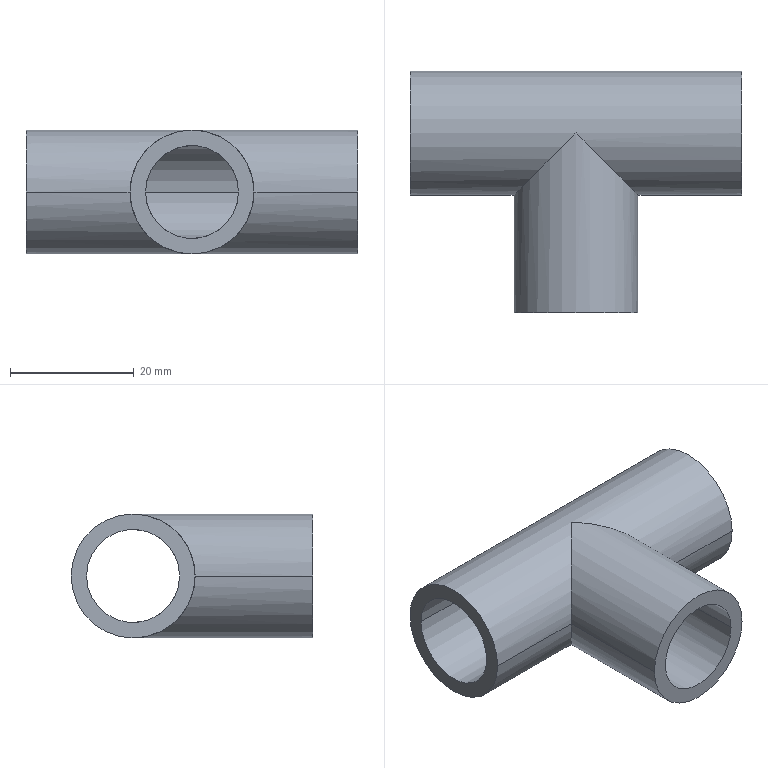Part | SolidWorks | features ICE 2, Sweep 2 | 1 solid | 15 faces | box 53.5 x 39 x 20 mm | volume 9797 mm3 | cylinder 10 | plane 5 | commonest cylinder face diameters 15 x6 20 x4
STEP:
#1=CARTESIAN_POINT('',(-26.75,-7.5,0.));
#2=VERTEX_POINT('',#1);
#3=CARTESIAN_POINT('',(-26.75,7.5,0.));
#4=VERTEX_POINT('',#3);
#5=CARTESIAN_POINT('',(-26.75,0.,0.));
#6=DIRECTION('',(1.,0.,0.));
#7=DIRECTION('',(0.,1.,0.));
#8=AXIS2_PLACEMENT_3D('',#5,#6,#7);
#9=CIRCLE('',#8,7.5);
#10=EDGE_CURVE('',#2,#4,#9,.T.);
#11=ORIENTED_EDGE('',*,*,#10,.F.);
#12=CARTESIAN_POINT('',(-7.5,-7.5,0.));
#13=VERTEX_POINT('',#12);
#14=CARTESIAN_POINT('',(-26.75,-7.5,0.));
#15=DIRECTION('',(1.,0.,0.));
#16=VECTOR('',#15,1000.);
#17=LINE('',#14,#16);
#18=EDGE_CURVE('',#2,#13,#17,.T.);
#19=ORIENTED_EDGE('',*,*,#18,.T.);
#20=CARTESIAN_POINT('',(0.,0.,-7.5));
#21=VERTEX_POINT('',#20);
#22=CARTESIAN_POINT('',(-7.5,-7.5,0.));
#23=CARTESIAN_POINT('',(-7.5,-7.5,-4.393));
#24=CARTESIAN_POINT('',(-4.393,-4.393,-7.5));
#25=CARTESIAN_POINT('',(0.,0.,-7.5));
#26=(BOUNDED_CURVE()B_SPLINE_CURVE(3,(#22,#23,#24,#25),.UNSPECIFIED.,.F.,.F.)B_SPLINE_CURVE_WITH_KNOTS((4,4),(3.142,4.712),.UNSPECIFIED.)CURVE()GEOMETRIC_REPRESENTATION_ITEM()RATIONAL_B_SPLINE_CURVE((1.,0.8047,0.8047,1.))REPRESENTATION_ITEM(''));
#27=EDGE_CURVE('',#13,#21,#26,.T.);
#28=ORIENTED_EDGE('',*,*,#27,.T.);
#29=CARTESIAN_POINT('',(-1.,1.,-7.433));
#30=VERTEX_POINT('',#29);
#31=CARTESIAN_POINT('',(0.,0.,-7.5));
#32=CARTESIAN_POINT('',(-0.3346,0.3346,-7.5));
#33=CARTESIAN_POINT('',(-0.6684,0.6684,-7.478));
#34=CARTESIAN_POINT('',(-1.,1.,-7.433));
#35=(BOUNDED_CURVE()B_SPLINE_CURVE(3,(#31,#32,#33,#34),.UNSPECIFIED.,.F.,.F.)B_SPLINE_CURVE_WITH_KNOTS((4,4),(1.571,1.705),.UNSPECIFIED.)CURVE()GEOMETRIC_REPRESENTATION_ITEM()RATIONAL_B_SPLINE_CURVE((1.,0.9985,0.9985,1.))REPRESENTATION_ITEM(''));
#36=EDGE_CURVE('',#21,#30,#35,.T.);
#37=ORIENTED_EDGE('',*,*,#36,.T.);
#38=CARTESIAN_POINT('',(1.,1.,-7.433));
#39=VERTEX_POINT('',#38);
#40=CARTESIAN_POINT('',(-26.75,1.,-7.433));
#41=DIRECTION('',(-1.,0.,0.));
#42=VECTOR('',#41,1000.);
#43=LINE('',#40,#42);
#44=EDGE_CURVE('',#39,#30,#43,.T.);
#45=ORIENTED_EDGE('',*,*,#44,.F.);
#46=CARTESIAN_POINT('',(1.,1.,-7.433));
#47=CARTESIAN_POINT('',(0.6684,0.6684,-7.478));
#48=CARTESIAN_POINT('',(0.3346,0.3346,-7.5));
#49=CARTESIAN_POINT('',(0.,0.,-7.5));
#50=(BOUNDED_CURVE()B_SPLINE_CURVE(3,(#46,#47,#48,#49),.UNSPECIFIED.,.F.,.F.)B_SPLINE_CURVE_WITH_KNOTS((4,4),(1.437,1.571),.UNSPECIFIED.)CURVE()GEOMETRIC_REPRESENTATION_ITEM()RATIONAL_B_SPLINE_CURVE((1.,0.9985,0.9985,1.))REPRESENTATION_ITEM(''));
#51=EDGE_CURVE('',#39,#21,#50,.T.);
#52=ORIENTED_EDGE('',*,*,#51,.T.);
#53=CARTESIAN_POINT('',(7.5,-7.5,0.));
#54=VERTEX_POINT('',#53);
#55=CARTESIAN_POINT('',(0.,0.,-7.5));
#56=CARTESIAN_POINT('',(4.393,-4.393,-7.5));
#57=CARTESIAN_POINT('',(7.5,-7.5,-4.393));
#58=CARTESIAN_POINT('',(7.5,-7.5,0.));
#59=(BOUNDED_CURVE()B_SPLINE_CURVE(3,(#55,#56,#57,#58),.UNSPECIFIED.,.F.,.F.)B_SPLINE_CURVE_WITH_KNOTS((4,4),(4.712,6.283),.UNSPECIFIED.)CURVE()GEOMETRIC_REPRESENTATION_ITEM()RATIONAL_B_SPLINE_CURVE((1.,0.8047,0.8047,1.))REPRESENTATION_ITEM(''));
#60=EDGE_CURVE('',#21,#54,#59,.T.);
#61=ORIENTED_EDGE('',*,*,#60,.T.);
#62=CARTESIAN_POINT('',(26.75,-7.5,0.));
#63=VERTEX_POINT('',#62);
#64=CARTESIAN_POINT('',(-26.75,-7.5,0.));
#65=DIRECTION('',(1.,0.,0.));
#66=VECTOR('',#65,1000.);
#67=LINE('',#64,#66);
#68=EDGE_CURVE('',#54,#63,#67,.T.);
#69=ORIENTED_EDGE('',*,*,#68,.T.);
#70=CARTESIAN_POINT('',(26.75,7.5,0.));
#71=VERTEX_POINT('',#70);
#72=CARTESIAN_POINT('',(26.75,0.,0.));
#73=DIRECTION('',(1.,0.,0.));
#74=DIRECTION('',(0.,1.,0.));
#75=AXIS2_PLACEMENT_3D('',#72,#73,#74);
#76=CIRCLE('',#75,7.5);
#77=EDGE_CURVE('',#63,#71,#76,.T.);
#78=ORIENTED_EDGE('',*,*,#77,.T.);
#79=CARTESIAN_POINT('',(-26.75,7.5,0.));
#80=DIRECTION('',(1.,0.,0.));
#81=VECTOR('',#80,1000.);
#82=LINE('',#79,#81);
#83=EDGE_CURVE('',#4,#71,#82,.T.);
#84=ORIENTED_EDGE('',*,*,#83,.F.);
#85=EDGE_LOOP('',(#11,#19,#28,#37,#45,#52,#61,#69,#78,#84));
#86=FACE_OUTER_BOUND('',#85,.T.);
#87=CARTESIAN_POINT('',(-26.75,0.,0.));
#88=DIRECTION('',(1.,0.,0.));
#89=DIRECTION('',(0.,1.,0.));
#90=AXIS2_PLACEMENT_3D('',#87,#88,#89);
#91=CYLINDRICAL_SURFACE('',#90,7.5);
#92=ADVANCED_FACE('',(#86),#91,.F.);
#93=ORIENTED_EDGE('',*,*,#27,.F.);
#94=CARTESIAN_POINT('',(-7.5,-29.,0.));
#95=VERTEX_POINT('',#94);
#96=CARTESIAN_POINT('',(-7.5,0.,0.));
#97=DIRECTION('',(0.,-1.,0.));
#98=VECTOR('',#97,1000.);
#99=LINE('',#96,#98);
#100=EDGE_CURVE('',#13,#95,#99,.T.);
#101=ORIENTED_EDGE('',*,*,#100,.T.);
#102=CARTESIAN_POINT('',(7.5,-29.,0.));
#103=VERTEX_POINT('',#102);
#104=CARTESIAN_POINT('',(0.,-29.,0.));
#105=DIRECTION('',(0.,-1.,0.));
#106=DIRECTION('',(1.,0.,0.));
#107=AXIS2_PLACEMENT_3D('',#104,#105,#106);
#108=CIRCLE('',#107,7.5);
#109=EDGE_CURVE('',#95,#103,#108,.T.);
#110=ORIENTED_EDGE('',*,*,#109,.T.);
#111=CARTESIAN_POINT('',(7.5,0.,0.));
#112=DIRECTION('',(0.,-1.,0.));
#113=VECTOR('',#112,1000.);
#114=LINE('',#111,#113);
#115=EDGE_CURVE('',#54,#103,#114,.T.);
#116=ORIENTED_EDGE('',*,*,#115,.F.);
#117=ORIENTED_EDGE('',*,*,#60,.F.);
#118=EDGE_LOOP('',(#93,#101,#110,#116,#117));
#119=FACE_OUTER_BOUND('',#118,.T.);
#120=CARTESIAN_POINT('',(0.,0.,0.));
#121=DIRECTION('',(0.,-1.,0.));
#122=DIRECTION('',(1.,0.,0.));
#123=AXIS2_PLACEMENT_3D('',#120,#121,#122);
#124=CYLINDRICAL_SURFACE('',#123,7.5);
#125=ADVANCED_FACE('',(#119),#124,.F.);
#126=CARTESIAN_POINT('',(0.,0.,10.));
#127=VERTEX_POINT('',#126);
#128=CARTESIAN_POINT('',(-10.,-10.,0.));
#129=VERTEX_POINT('',#128);
#130=CARTESIAN_POINT('',(0.,0.,10.));
#131=CARTESIAN_POINT('',(-5.858,-5.858,10.));
#132=CARTESIAN_POINT('',(-10.,-10.,5.858));
#133=CARTESIAN_POINT('',(-10.,-10.,0.));
#134=(BOUNDED_CURVE()B_SPLINE_CURVE(3,(#130,#131,#132,#133),.UNSPECIFIED.,.F.,.F.)B_SPLINE_CURVE_WITH_KNOTS((4,4),(1.571,3.142),.UNSPECIFIED.)CURVE()GEOMETRIC_REPRESENTATION_ITEM()RATIONAL_B_SPLINE_CURVE((1.,0.8047,0.8047,1.))REPRESENTATION_ITEM(''));
#135=EDGE_CURVE('',#127,#129,#134,.T.);
#136=ORIENTED_EDGE('',*,*,#135,.T.);
#137=CARTESIAN_POINT('',(-10.,-29.,0.));
#138=VERTEX_POINT('',#137);
#139=CARTESIAN_POINT('',(-10.,0.,0.));
#140=DIRECTION('',(0.,-1.,0.));
#141=VECTOR('',#140,1000.);
#142=LINE('',#139,#141);
#143=EDGE_CURVE('',#129,#138,#142,.T.);
#144=ORIENTED_EDGE('',*,*,#143,.T.);
#145=CARTESIAN_POINT('',(10.,-29.,0.));
#146=VERTEX_POINT('',#145);
#147=CARTESIAN_POINT('',(0.,-29.,0.));
#148=DIRECTION('',(0.,-1.,0.));
#149=DIRECTION('',(1.,0.,0.));
#150=AXIS2_PLACEMENT_3D('',#147,#148,#149);
#151=CIRCLE('',#150,10.);
#152=EDGE_CURVE('',#146,#138,#151,.T.);
#153=ORIENTED_EDGE('',*,*,#152,.F.);
#154=CARTESIAN_POINT('',(10.,-10.,0.));
#155=VERTEX_POINT('',#154);
#156=CARTESIAN_POINT('',(10.,0.,0.));
#157=DIRECTION('',(0.,-1.,0.));
#158=VECTOR('',#157,1000.);
#159=LINE('',#156,#158);
#160=EDGE_CURVE('',#155,#146,#159,.T.);
#161=ORIENTED_EDGE('',*,*,#160,.F.);
#162=CARTESIAN_POINT('',(10.,-10.,0.));
#163=CARTESIAN_POINT('',(10.,-10.,5.858));
#164=CARTESIAN_POINT('',(5.858,-5.858,10.));
#165=CARTESIAN_POINT('',(0.,0.,10.));
#166=(BOUNDED_CURVE()B_SPLINE_CURVE(3,(#162,#163,#164,#165),.UNSPECIFIED.,.F.,.F.)B_SPLINE_CURVE_WITH_KNOTS((4,4),(0.,1.571),.UNSPECIFIED.)CURVE()GEOMETRIC_REPRESENTATION_ITEM()RATIONAL_B_SPLINE_CURVE((1.,0.8047,0.8047,1.))REPRESENTATION_ITEM(''));
#167=EDGE_CURVE('',#155,#127,#166,.T.);
#168=ORIENTED_EDGE('',*,*,#167,.T.);
#169=EDGE_LOOP('',(#136,#144,#153,#161,#168));
#170=FACE_OUTER_BOUND('',#169,.T.);
#171=CARTESIAN_POINT('',(0.,0.,0.));
#172=DIRECTION('',(0.,-1.,0.));
#173=DIRECTION('',(1.,0.,0.));
#174=AXIS2_PLACEMENT_3D('',#171,#172,#173);
#175=CYLINDRICAL_SURFACE('',#174,10.);
#176=ADVANCED_FACE('',(#170),#175,.T.);
#177=CARTESIAN_POINT('',(-26.75,10.,0.));
#178=VERTEX_POINT('',#177);
#179=CARTESIAN_POINT('',(-26.75,-10.,0.));
#180=VERTEX_POINT('',#179);
#181=CARTESIAN_POINT('',(-26.75,0.,0.));
#182=DIRECTION('',(1.,0.,0.));
#183=DIRECTION('',(0.,1.,0.));
#184=AXIS2_PLACEMENT_3D('',#181,#182,#183);
#185=CIRCLE('',#184,10.);
#186=EDGE_CURVE('',#178,#180,#185,.T.);
#187=ORIENTED_EDGE('',*,*,#186,.T.);
#188=CARTESIAN_POINT('',(-26.75,-10.,0.));
#189=DIRECTION('',(1.,0.,0.));
#190=VECTOR('',#189,1000.);
#191=LINE('',#188,#190);
#192=EDGE_CURVE('',#180,#129,#191,.T.);
#193=ORIENTED_EDGE('',*,*,#192,.T.);
#194=ORIENTED_EDGE('',*,*,#135,.F.);
#195=ORIENTED_EDGE('',*,*,#167,.F.);
#196=CARTESIAN_POINT('',(26.75,-10.,0.));
#197=VERTEX_POINT('',#196);
#198=CARTESIAN_POINT('',(-26.75,-10.,0.));
#199=DIRECTION('',(1.,0.,0.));
#200=VECTOR('',#199,1000.);
#201=LINE('',#198,#200);
#202=EDGE_CURVE('',#155,#197,#201,.T.);
#203=ORIENTED_EDGE('',*,*,#202,.T.);
#204=CARTESIAN_POINT('',(26.75,10.,0.));
#205=VERTEX_POINT('',#204);
#206=CARTESIAN_POINT('',(26.75,0.,0.));
#207=DIRECTION('',(1.,0.,0.));
#208=DIRECTION('',(0.,1.,0.));
#209=AXIS2_PLACEMENT_3D('',#206,#207,#208);
#210=CIRCLE('',#209,10.);
#211=EDGE_CURVE('',#205,#197,#210,.T.);
#212=ORIENTED_EDGE('',*,*,#211,.F.);
#213=CARTESIAN_POINT('',(-26.75,10.,0.));
#214=DIRECTION('',(1.,0.,0.));
#215=VECTOR('',#214,1000.);
#216=LINE('',#213,#215);
#217=EDGE_CURVE('',#178,#205,#216,.T.);
#218=ORIENTED_EDGE('',*,*,#217,.F.);
#219=EDGE_LOOP('',(#187,#193,#194,#195,#203,#212,#218));
#220=FACE_OUTER_BOUND('',#219,.T.);
#221=CARTESIAN_POINT('',(-26.75,0.,0.));
#222=DIRECTION('',(1.,0.,0.));
#223=DIRECTION('',(0.,1.,0.));
#224=AXIS2_PLACEMENT_3D('',#221,#222,#223);
#225=CYLINDRICAL_SURFACE('',#224,10.);
#226=ADVANCED_FACE('',(#220),#225,.T.);
#227=ORIENTED_EDGE('',*,*,#192,.F.);
#228=CARTESIAN_POINT('',(-26.75,0.,0.));
#229=DIRECTION('',(1.,0.,0.));
#230=DIRECTION('',(0.,1.,0.));
#231=AXIS2_PLACEMENT_3D('',#228,#229,#230);
#232=CIRCLE('',#231,10.);
#233=EDGE_CURVE('',#180,#178,#232,.T.);
#234=ORIENTED_EDGE('',*,*,#233,.T.);
#235=ORIENTED_EDGE('',*,*,#217,.T.);
#236=CARTESIAN_POINT('',(26.75,0.,0.));
#237=DIRECTION('',(1.,0.,0.));
#238=DIRECTION('',(0.,1.,0.));
#239=AXIS2_PLACEMENT_3D('',#236,#237,#238);
#240=CIRCLE('',#239,10.);
#241=EDGE_CURVE('',#197,#205,#240,.T.);
#242=ORIENTED_EDGE('',*,*,#241,.F.);
#243=ORIENTED_EDGE('',*,*,#202,.F.);
#244=CARTESIAN_POINT('',(0.,0.,-10.));
#245=VERTEX_POINT('',#244);
#246=CARTESIAN_POINT('',(0.,0.,-10.));
#247=CARTESIAN_POINT('',(5.858,-5.858,-10.));
#248=CARTESIAN_POINT('',(10.,-10.,-5.858));
#249=CARTESIAN_POINT('',(10.,-10.,0.));
#250=(BOUNDED_CURVE()B_SPLINE_CURVE(3,(#246,#247,#248,#249),.UNSPECIFIED.,.F.,.F.)B_SPLINE_CURVE_WITH_KNOTS((4,4),(4.712,6.283),.UNSPECIFIED.)CURVE()GEOMETRIC_REPRESENTATION_ITEM()RATIONAL_B_SPLINE_CURVE((1.,0.8047,0.8047,1.))REPRESENTATION_ITEM(''));
#251=EDGE_CURVE('',#245,#155,#250,.T.);
#252=ORIENTED_EDGE('',*,*,#251,.F.);
#253=CARTESIAN_POINT('',(-10.,-10.,0.));
#254=CARTESIAN_POINT('',(-10.,-10.,-5.858));
#255=CARTESIAN_POINT('',(-5.858,-5.858,-10.));
#256=CARTESIAN_POINT('',(0.,0.,-10.));
#257=(BOUNDED_CURVE()B_SPLINE_CURVE(3,(#253,#254,#255,#256),.UNSPECIFIED.,.F.,.F.)B_SPLINE_CURVE_WITH_KNOTS((4,4),(3.142,4.712),.UNSPECIFIED.)CURVE()GEOMETRIC_REPRESENTATION_ITEM()RATIONAL_B_SPLINE_CURVE((1.,0.8047,0.8047,1.))REPRESENTATION_ITEM(''));
#258=EDGE_CURVE('',#129,#245,#257,.T.);
#259=ORIENTED_EDGE('',*,*,#258,.F.);
#260=EDGE_LOOP('',(#227,#234,#235,#242,#243,#252,#259));
#261=FACE_OUTER_BOUND('',#260,.T.);
#262=CARTESIAN_POINT('',(-26.75,0.,0.));
#263=DIRECTION('',(1.,0.,0.));
#264=DIRECTION('',(0.,1.,0.));
#265=AXIS2_PLACEMENT_3D('',#262,#263,#264);
#266=CYLINDRICAL_SURFACE('',#265,10.);
#267=ADVANCED_FACE('',(#261),#266,.T.);
#268=CARTESIAN_POINT('',(26.75,0.,0.));
#269=DIRECTION('',(1.,0.,0.));
#270=DIRECTION('',(0.,1.,0.));
#271=AXIS2_PLACEMENT_3D('',#268,#269,#270);
#272=CIRCLE('',#271,7.5);
#273=EDGE_CURVE('',#71,#63,#272,.T.);
#274=ORIENTED_EDGE('',*,*,#273,.F.);
#275=ORIENTED_EDGE('',*,*,#77,.F.);
#276=EDGE_LOOP('',(#274,#275));
#277=FACE_BOUND('',#276,.T.);
#278=ORIENTED_EDGE('',*,*,#211,.T.);
#279=ORIENTED_EDGE('',*,*,#241,.T.);
#280=EDGE_LOOP('',(#278,#279));
#281=FACE_OUTER_BOUND('',#280,.T.);
#282=CARTESIAN_POINT('',(26.75,0.,0.));
#283=DIRECTION('',(1.,0.,0.));
#284=DIRECTION('',(0.,1.,0.));
#285=AXIS2_PLACEMENT_3D('',#282,#283,#284);
#286=PLANE('',#285);
#287=ADVANCED_FACE('',(#277,#281),#286,.T.);
#288=CARTESIAN_POINT('',(-26.75,0.,0.));
#289=DIRECTION('',(1.,0.,0.));
#290=DIRECTION('',(0.,1.,0.));
#291=AXIS2_PLACEMENT_3D('',#288,#289,#290);
#292=CIRCLE('',#291,7.5);
#293=EDGE_CURVE('',#4,#2,#292,.T.);
#294=ORIENTED_EDGE('',*,*,#293,.T.);
#295=ORIENTED_EDGE('',*,*,#10,.T.);
#296=EDGE_LOOP('',(#294,#295));
#297=FACE_BOUND('',#296,.T.);
#298=ORIENTED_EDGE('',*,*,#186,.F.);
#299=ORIENTED_EDGE('',*,*,#233,.F.);
#300=EDGE_LOOP('',(#298,#299));
#301=FACE_OUTER_BOUND('',#300,.T.);
#302=CARTESIAN_POINT('',(-26.75,0.,0.));
#303=DIRECTION('',(1.,0.,0.));
#304=DIRECTION('',(0.,1.,0.));
#305=AXIS2_PLACEMENT_3D('',#302,#303,#304);
#306=PLANE('',#305);
#307=ADVANCED_FACE('',(#297,#301),#306,.F.);
#308=ORIENTED_EDGE('',*,*,#143,.F.);
#309=ORIENTED_EDGE('',*,*,#258,.T.);
#310=ORIENTED_EDGE('',*,*,#251,.T.);
#311=ORIENTED_EDGE('',*,*,#160,.T.);
#312=CARTESIAN_POINT('',(0.,-29.,0.));
#313=DIRECTION('',(0.,-1.,0.));
#314=DIRECTION('',(1.,0.,0.));
#315=AXIS2_PLACEMENT_3D('',#312,#313,#314);
#316=CIRCLE('',#315,10.);
#317=EDGE_CURVE('',#138,#146,#316,.T.);
#318=ORIENTED_EDGE('',*,*,#317,.F.);
#319=EDGE_LOOP('',(#308,#309,#310,#311,#318));
#320=FACE_OUTER_BOUND('',#319,.T.);
#321=CARTESIAN_POINT('',(0.,0.,0.));
#322=DIRECTION('',(0.,-1.,0.));
#323=DIRECTION('',(1.,0.,0.));
#324=AXIS2_PLACEMENT_3D('',#321,#322,#323);
#325=CYLINDRICAL_SURFACE('',#324,10.);
#326=ADVANCED_FACE('',(#320),#325,.T.);
#327=CARTESIAN_POINT('',(0.,-29.,0.));
#328=DIRECTION('',(0.,-1.,0.));
#329=DIRECTION('',(1.,0.,0.));
#330=AXIS2_PLACEMENT_3D('',#327,#328,#329);
#331=CIRCLE('',#330,7.5);
#332=EDGE_CURVE('',#103,#95,#331,.T.);
#333=ORIENTED_EDGE('',*,*,#332,.F.);
#334=ORIENTED_EDGE('',*,*,#109,.F.);
#335=EDGE_LOOP('',(#333,#334));
#336=FACE_BOUND('',#335,.T.);
#337=ORIENTED_EDGE('',*,*,#152,.T.);
#338=ORIENTED_EDGE('',*,*,#317,.T.);
#339=EDGE_LOOP('',(#337,#338));
#340=FACE_OUTER_BOUND('',#339,.T.);
#341=CARTESIAN_POINT('',(0.,-29.,0.));
#342=DIRECTION('',(0.,-1.,0.));
#343=DIRECTION('',(1.,0.,0.));
#344=AXIS2_PLACEMENT_3D('',#341,#342,#343);
#345=PLANE('',#344);
#346=ADVANCED_FACE('',(#336,#340),#345,.T.);
#347=ORIENTED_EDGE('',*,*,#100,.F.);
#348=CARTESIAN_POINT('',(0.,0.,7.5));
#349=VERTEX_POINT('',#348);
#350=CARTESIAN_POINT('',(0.,0.,7.5));
#351=CARTESIAN_POINT('',(-4.393,-4.393,7.5));
#352=CARTESIAN_POINT('',(-7.5,-7.5,4.393));
#353=CARTESIAN_POINT('',(-7.5,-7.5,0.));
#354=(BOUNDED_CURVE()B_SPLINE_CURVE(3,(#350,#351,#352,#353),.UNSPECIFIED.,.F.,.F.)B_SPLINE_CURVE_WITH_KNOTS((4,4),(1.571,3.142),.UNSPECIFIED.)CURVE()GEOMETRIC_REPRESENTATION_ITEM()RATIONAL_B_SPLINE_CURVE((1.,0.8047,0.8047,1.))REPRESENTATION_ITEM(''));
#355=EDGE_CURVE('',#349,#13,#354,.T.);
#356=ORIENTED_EDGE('',*,*,#355,.F.);
#357=CARTESIAN_POINT('',(7.5,-7.5,0.));
#358=CARTESIAN_POINT('',(7.5,-7.5,4.393));
#359=CARTESIAN_POINT('',(4.393,-4.393,7.5));
#360=CARTESIAN_POINT('',(0.,0.,7.5));
#361=(BOUNDED_CURVE()B_SPLINE_CURVE(3,(#357,#358,#359,#360),.UNSPECIFIED.,.F.,.F.)B_SPLINE_CURVE_WITH_KNOTS((4,4),(0.,1.571),.UNSPECIFIED.)CURVE()GEOMETRIC_REPRESENTATION_ITEM()RATIONAL_B_SPLINE_CURVE((1.,0.8047,0.8047,1.))REPRESENTATION_ITEM(''));
#362=EDGE_CURVE('',#54,#349,#361,.T.);
#363=ORIENTED_EDGE('',*,*,#362,.F.);
#364=ORIENTED_EDGE('',*,*,#115,.T.);
#365=ORIENTED_EDGE('',*,*,#332,.T.);
#366=EDGE_LOOP('',(#347,#356,#363,#364,#365));
#367=FACE_OUTER_BOUND('',#366,.T.);
#368=CARTESIAN_POINT('',(0.,0.,0.));
#369=DIRECTION('',(0.,-1.,0.));
#370=DIRECTION('',(1.,0.,0.));
#371=AXIS2_PLACEMENT_3D('',#368,#369,#370);
#372=CYLINDRICAL_SURFACE('',#371,7.5);
#373=ADVANCED_FACE('',(#367),#372,.F.);
#374=ORIENTED_EDGE('',*,*,#18,.F.);
#375=ORIENTED_EDGE('',*,*,#293,.F.);
#376=ORIENTED_EDGE('',*,*,#83,.T.);
#377=ORIENTED_EDGE('',*,*,#273,.T.);
#378=ORIENTED_EDGE('',*,*,#68,.F.);
#379=ORIENTED_EDGE('',*,*,#362,.T.);
#380=CARTESIAN_POINT('',(1.,1.,7.433));
#381=VERTEX_POINT('',#380);
#382=CARTESIAN_POINT('',(0.,0.,7.5));
#383=CARTESIAN_POINT('',(0.3346,0.3346,7.5));
#384=CARTESIAN_POINT('',(0.6684,0.6684,7.478));
#385=CARTESIAN_POINT('',(1.,1.,7.433));
#386=(BOUNDED_CURVE()B_SPLINE_CURVE(3,(#382,#383,#384,#385),.UNSPECIFIED.,.F.,.F.)B_SPLINE_CURVE_WITH_KNOTS((4,4),(4.712,4.846),.UNSPECIFIED.)CURVE()GEOMETRIC_REPRESENTATION_ITEM()RATIONAL_B_SPLINE_CURVE((1.,0.9985,0.9985,1.))REPRESENTATION_ITEM(''));
#387=EDGE_CURVE('',#349,#381,#386,.T.);
#388=ORIENTED_EDGE('',*,*,#387,.T.);
#389=CARTESIAN_POINT('',(-1.,1.,7.433));
#390=VERTEX_POINT('',#389);
#391=CARTESIAN_POINT('',(-26.75,1.,7.433));
#392=DIRECTION('',(1.,0.,0.));
#393=VECTOR('',#392,1000.);
#394=LINE('',#391,#393);
#395=EDGE_CURVE('',#390,#381,#394,.T.);
#396=ORIENTED_EDGE('',*,*,#395,.F.);
#397=CARTESIAN_POINT('',(-1.,1.,7.433));
#398=CARTESIAN_POINT('',(-0.6684,0.6684,7.478));
#399=CARTESIAN_POINT('',(-0.3346,0.3346,7.5));
#400=CARTESIAN_POINT('',(0.,0.,7.5));
#401=(BOUNDED_CURVE()B_SPLINE_CURVE(3,(#397,#398,#399,#400),.UNSPECIFIED.,.F.,.F.)B_SPLINE_CURVE_WITH_KNOTS((4,4),(4.579,4.712),.UNSPECIFIED.)CURVE()GEOMETRIC_REPRESENTATION_ITEM()RATIONAL_B_SPLINE_CURVE((1.,0.9985,0.9985,1.))REPRESENTATION_ITEM(''));
#402=EDGE_CURVE('',#390,#349,#401,.T.);
#403=ORIENTED_EDGE('',*,*,#402,.T.);
#404=ORIENTED_EDGE('',*,*,#355,.T.);
#405=EDGE_LOOP('',(#374,#375,#376,#377,#378,#379,#388,#396,#403,#404));
#406=FACE_OUTER_BOUND('',#405,.T.);
#407=CARTESIAN_POINT('',(-26.75,0.,0.));
#408=DIRECTION('',(1.,0.,0.));
#409=DIRECTION('',(0.,1.,0.));
#410=AXIS2_PLACEMENT_3D('',#407,#408,#409);
#411=CYLINDRICAL_SURFACE('',#410,7.5);
#412=ADVANCED_FACE('',(#406),#411,.F.);
#413=ORIENTED_EDGE('',*,*,#395,.T.);
#414=CARTESIAN_POINT('',(0.,1.,0.));
#415=DIRECTION('',(0.,-1.,0.));
#416=DIRECTION('',(1.,0.,0.));
#417=AXIS2_PLACEMENT_3D('',#414,#415,#416);
#418=CIRCLE('',#417,7.5);
#419=EDGE_CURVE('',#381,#390,#418,.T.);
#420=ORIENTED_EDGE('',*,*,#419,.T.);
#421=EDGE_LOOP('',(#413,#420));
#422=FACE_OUTER_BOUND('',#421,.T.);
#423=CARTESIAN_POINT('',(0.,1.,0.));
#424=DIRECTION('',(0.,-1.,0.));
#425=DIRECTION('',(1.,0.,0.));
#426=AXIS2_PLACEMENT_3D('',#423,#424,#425);
#427=PLANE('',#426);
#428=ADVANCED_FACE('',(#422),#427,.T.);
#429=ORIENTED_EDGE('',*,*,#402,.F.);
#430=ORIENTED_EDGE('',*,*,#419,.F.);
#431=ORIENTED_EDGE('',*,*,#387,.F.);
#432=EDGE_LOOP('',(#429,#430,#431));
#433=FACE_OUTER_BOUND('',#432,.T.);
#434=CARTESIAN_POINT('',(0.,1.,0.));
#435=DIRECTION('',(0.,-1.,0.));
#436=DIRECTION('',(1.,0.,0.));
#437=AXIS2_PLACEMENT_3D('',#434,#435,#436);
#438=CYLINDRICAL_SURFACE('',#437,7.5);
#439=ADVANCED_FACE('',(#433),#438,.F.);
#440=ORIENTED_EDGE('',*,*,#44,.T.);
#441=CARTESIAN_POINT('',(0.,1.,0.));
#442=DIRECTION('',(0.,-1.,0.));
#443=DIRECTION('',(1.,0.,0.));
#444=AXIS2_PLACEMENT_3D('',#441,#442,#443);
#445=CIRCLE('',#444,7.5);
#446=EDGE_CURVE('',#30,#39,#445,.T.);
#447=ORIENTED_EDGE('',*,*,#446,.T.);
#448=EDGE_LOOP('',(#440,#447));
#449=FACE_OUTER_BOUND('',#448,.T.);
#450=CARTESIAN_POINT('',(0.,1.,0.));
#451=DIRECTION('',(0.,-1.,0.));
#452=DIRECTION('',(1.,0.,0.));
#453=AXIS2_PLACEMENT_3D('',#450,#451,#452);
#454=PLANE('',#453);
#455=ADVANCED_FACE('',(#449),#454,.T.);
#456=ORIENTED_EDGE('',*,*,#446,.F.);
#457=ORIENTED_EDGE('',*,*,#36,.F.);
#458=ORIENTED_EDGE('',*,*,#51,.F.);
#459=EDGE_LOOP('',(#456,#457,#458));
#460=FACE_OUTER_BOUND('',#459,.T.);
#461=CARTESIAN_POINT('',(0.,1.,0.));
#462=DIRECTION('',(0.,-1.,0.));
#463=DIRECTION('',(1.,0.,0.));
#464=AXIS2_PLACEMENT_3D('',#461,#462,#463);
#465=CYLINDRICAL_SURFACE('',#464,7.5);
#466=ADVANCED_FACE('',(#460),#465,.F.);
#467=CLOSED_SHELL('',(#92,#125,#176,#226,#267,#287,#307,#326,#346,#373,#412,#428,#439,#455,#466));
#468=MANIFOLD_SOLID_BREP('',#467);
#469=CARTESIAN_POINT('',(0.,0.,0.));
#470=DIRECTION('',(0.,0.,1.));
#471=DIRECTION('',(1.,0.,0.));
#472=AXIS2_PLACEMENT_3D('',#469,#470,#471);
#473=(LENGTH_UNIT()NAMED_UNIT(*)SI_UNIT(.MILLI.,.METRE.));
#474=UNCERTAINTY_MEASURE_WITH_UNIT(LENGTH_MEASURE(0.00001),#473,'','');
#475=(NAMED_UNIT(*)PLANE_ANGLE_UNIT()SI_UNIT($,.RADIAN.));
#476=(NAMED_UNIT(*)SI_UNIT($,.STERADIAN.)SOLID_ANGLE_UNIT());
#477=(GEOMETRIC_REPRESENTATION_CONTEXT(3)GLOBAL_UNCERTAINTY_ASSIGNED_CONTEXT((#474))GLOBAL_UNIT_ASSIGNED_CONTEXT((#473,#475,#476))REPRESENTATION_CONTEXT('',''));
#478=ADVANCED_BREP_SHAPE_REPRESENTATION('',(#468,#472),#477);